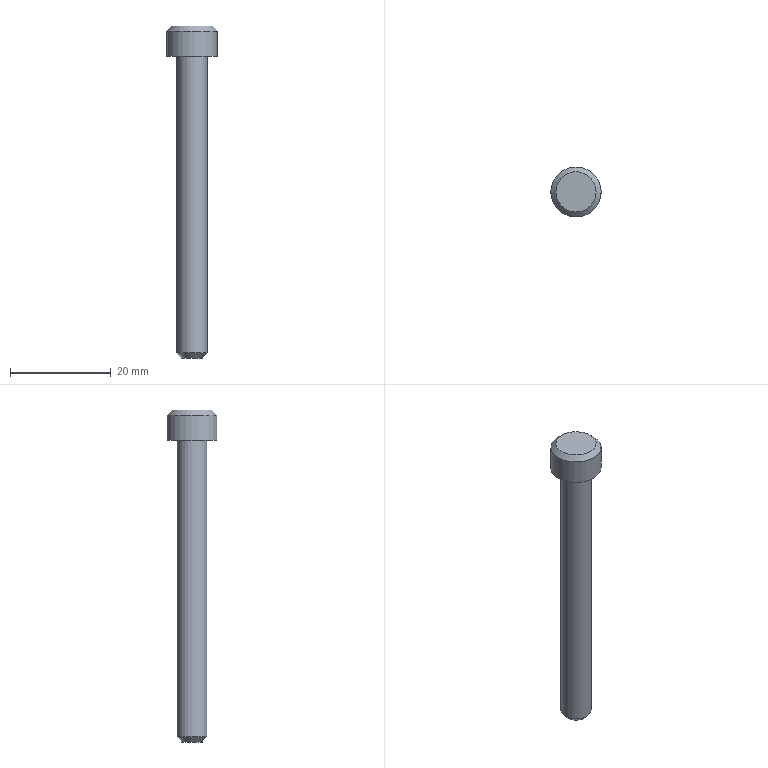Part | NX | features PG_666 2 | 1 solid | 7 faces | box 10 x 10 x 66 mm | volume 2149 mm3 | plane 3 | cylinder 2 | cone 2 | commonest cylinder face diameters 6.007 x1 10 x1
STEP:
#1=CARTESIAN_POINT('',(3909.09,-923.622,794.716));
#2=VERTEX_POINT('',#1);
#3=CARTESIAN_POINT('',(3912.094,-923.622,794.716));
#4=DIRECTION('',(0.,0.,-1.));
#5=DIRECTION('',(-1.,0.,0.));
#6=AXIS2_PLACEMENT_3D('',#3,#4,#5);
#7=CIRCLE('',#6,3.003);
#8=EDGE_CURVE('',#2,#2,#7,.F.);
#9=ORIENTED_EDGE('',*,*,#8,.T.);
#10=EDGE_LOOP('',(#9));
#11=FACE_BOUND('',#10,.T.);
#12=CARTESIAN_POINT('',(3909.09,-923.622,853.716));
#13=VERTEX_POINT('',#12);
#14=CARTESIAN_POINT('',(3912.094,-923.622,853.716));
#15=DIRECTION('',(0.,0.,-1.));
#16=DIRECTION('',(-1.,0.,0.));
#17=AXIS2_PLACEMENT_3D('',#14,#15,#16);
#18=CIRCLE('',#17,3.003);
#19=EDGE_CURVE('',#13,#13,#18,.F.);
#20=ORIENTED_EDGE('',*,*,#19,.F.);
#21=EDGE_LOOP('',(#20));
#22=FACE_BOUND('',#21,.T.);
#23=CARTESIAN_POINT('',(3912.094,-923.622,823.716));
#24=DIRECTION('',(0.,0.,1.));
#25=DIRECTION('',(1.,0.,0.));
#26=AXIS2_PLACEMENT_3D('',#23,#24,#25);
#27=CYLINDRICAL_SURFACE('',#26,3.003);
#28=ADVANCED_FACE('',(#11,#22),#27,.T.);
#29=CARTESIAN_POINT('',(3910.09,-923.622,793.716));
#30=VERTEX_POINT('',#29);
#31=CARTESIAN_POINT('',(3912.094,-923.622,793.716));
#32=DIRECTION('',(0.,0.,-1.));
#33=DIRECTION('',(-1.,0.,0.));
#34=AXIS2_PLACEMENT_3D('',#31,#32,#33);
#35=CIRCLE('',#34,2.003);
#36=EDGE_CURVE('',#30,#30,#35,.T.);
#37=ORIENTED_EDGE('',*,*,#36,.T.);
#38=EDGE_LOOP('',(#37));
#39=FACE_BOUND('',#38,.T.);
#40=CARTESIAN_POINT('',(3912.094,-923.622,793.716));
#41=DIRECTION('',(0.,0.,-1.));
#42=DIRECTION('',(-1.,0.,0.));
#43=AXIS2_PLACEMENT_3D('',#40,#41,#42);
#44=PLANE('',#43);
#45=ADVANCED_FACE('',(#39),#44,.T.);
#46=CARTESIAN_POINT('',(3916.094,-923.622,859.716));
#47=VERTEX_POINT('',#46);
#48=CARTESIAN_POINT('',(3912.094,-923.622,859.716));
#49=DIRECTION('',(0.,0.,1.));
#50=DIRECTION('',(1.,0.,0.));
#51=AXIS2_PLACEMENT_3D('',#48,#49,#50);
#52=CIRCLE('',#51,4.);
#53=EDGE_CURVE('',#47,#47,#52,.T.);
#54=ORIENTED_EDGE('',*,*,#53,.T.);
#55=EDGE_LOOP('',(#54));
#56=FACE_BOUND('',#55,.T.);
#57=CARTESIAN_POINT('',(3912.094,-923.622,859.716));
#58=DIRECTION('',(0.,0.,1.));
#59=DIRECTION('',(1.,0.,0.));
#60=AXIS2_PLACEMENT_3D('',#57,#58,#59);
#61=PLANE('',#60);
#62=ADVANCED_FACE('',(#56),#61,.T.);
#63=ORIENTED_EDGE('',*,*,#19,.T.);
#64=EDGE_LOOP('',(#63));
#65=FACE_BOUND('',#64,.T.);
#66=CARTESIAN_POINT('',(3917.094,-923.622,853.716));
#67=VERTEX_POINT('',#66);
#68=CARTESIAN_POINT('',(3912.094,-923.622,853.716));
#69=DIRECTION('',(0.,0.,1.));
#70=DIRECTION('',(1.,0.,0.));
#71=AXIS2_PLACEMENT_3D('',#68,#69,#70);
#72=CIRCLE('',#71,5.);
#73=EDGE_CURVE('',#67,#67,#72,.T.);
#74=ORIENTED_EDGE('',*,*,#73,.F.);
#75=EDGE_LOOP('',(#74));
#76=FACE_BOUND('',#75,.T.);
#77=CARTESIAN_POINT('',(3912.094,-923.622,853.716));
#78=DIRECTION('',(0.,0.,-1.));
#79=DIRECTION('',(-1.,0.,0.));
#80=AXIS2_PLACEMENT_3D('',#77,#78,#79);
#81=PLANE('',#80);
#82=ADVANCED_FACE('',(#65,#76),#81,.T.);
#83=CARTESIAN_POINT('',(3917.094,-923.622,858.716));
#84=VERTEX_POINT('',#83);
#85=CARTESIAN_POINT('',(3912.094,-923.622,858.716));
#86=DIRECTION('',(0.,0.,1.));
#87=DIRECTION('',(1.,0.,0.));
#88=AXIS2_PLACEMENT_3D('',#85,#86,#87);
#89=CIRCLE('',#88,5.);
#90=EDGE_CURVE('',#84,#84,#89,.F.);
#91=ORIENTED_EDGE('',*,*,#90,.T.);
#92=EDGE_LOOP('',(#91));
#93=FACE_BOUND('',#92,.T.);
#94=ORIENTED_EDGE('',*,*,#73,.T.);
#95=EDGE_LOOP('',(#94));
#96=FACE_BOUND('',#95,.T.);
#97=CARTESIAN_POINT('',(3912.094,-923.622,853.716));
#98=DIRECTION('',(0.,0.,1.));
#99=DIRECTION('',(1.,0.,0.));
#100=AXIS2_PLACEMENT_3D('',#97,#98,#99);
#101=CYLINDRICAL_SURFACE('',#100,5.);
#102=ADVANCED_FACE('',(#93,#96),#101,.T.);
#103=ORIENTED_EDGE('',*,*,#36,.F.);
#104=EDGE_LOOP('',(#103));
#105=FACE_BOUND('',#104,.T.);
#106=ORIENTED_EDGE('',*,*,#8,.F.);
#107=EDGE_LOOP('',(#106));
#108=FACE_BOUND('',#107,.T.);
#109=CARTESIAN_POINT('',(3912.094,-923.622,794.716));
#110=DIRECTION('',(0.,0.,1.));
#111=DIRECTION('',(1.,0.,0.));
#112=AXIS2_PLACEMENT_3D('',#109,#110,#111);
#113=CONICAL_SURFACE('',#112,3.003,0.7854);
#114=ADVANCED_FACE('',(#105,#108),#113,.T.);
#115=ORIENTED_EDGE('',*,*,#53,.F.);
#116=EDGE_LOOP('',(#115));
#117=FACE_BOUND('',#116,.T.);
#118=ORIENTED_EDGE('',*,*,#90,.F.);
#119=EDGE_LOOP('',(#118));
#120=FACE_BOUND('',#119,.T.);
#121=CARTESIAN_POINT('',(3912.094,-923.622,858.716));
#122=DIRECTION('',(0.,0.,-1.));
#123=DIRECTION('',(-1.,0.,0.));
#124=AXIS2_PLACEMENT_3D('',#121,#122,#123);
#125=CONICAL_SURFACE('',#124,5.,0.7854);
#126=ADVANCED_FACE('',(#117,#120),#125,.T.);
#127=CLOSED_SHELL('',(#28,#45,#62,#82,#102,#114,#126));
#128=MANIFOLD_SOLID_BREP('',#127);
#129=(LENGTH_UNIT()NAMED_UNIT(*)SI_UNIT(.MILLI.,.METRE.));
#130=UNCERTAINTY_MEASURE_WITH_UNIT(LENGTH_MEASURE(0.00001),#129,'','');
#131=(NAMED_UNIT(*)PLANE_ANGLE_UNIT()SI_UNIT($,.RADIAN.));
#132=(NAMED_UNIT(*)SI_UNIT($,.STERADIAN.)SOLID_ANGLE_UNIT());
#133=(GEOMETRIC_REPRESENTATION_CONTEXT(3)GLOBAL_UNCERTAINTY_ASSIGNED_CONTEXT((#130))GLOBAL_UNIT_ASSIGNED_CONTEXT((#129,#131,#132))REPRESENTATION_CONTEXT('',''));
#134=ADVANCED_BREP_SHAPE_REPRESENTATION('',(#128),#133);